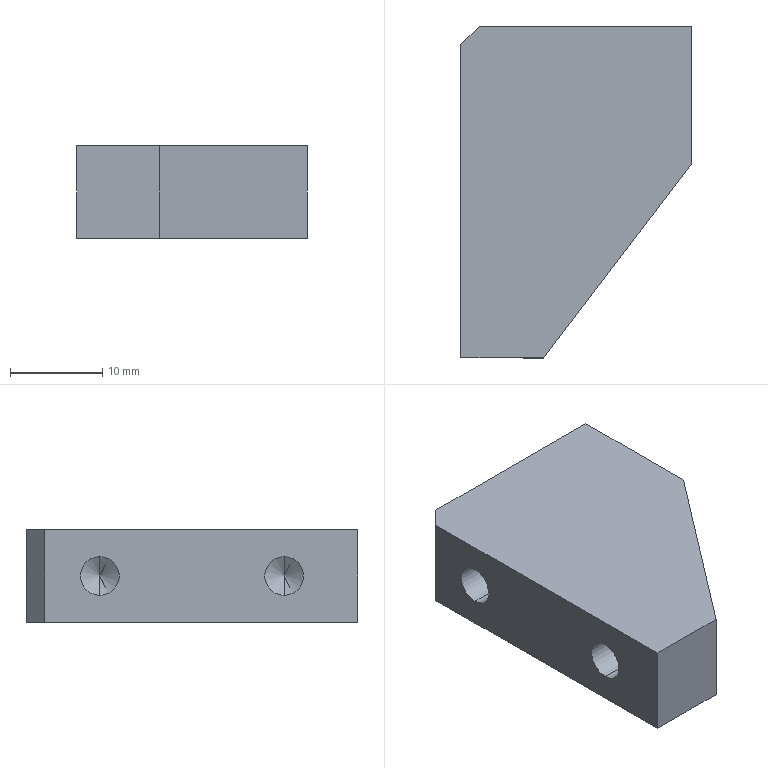Part | SolidWorks | features HoleWzd 2, Chamfer 1, Extrusion 1 | 1 solid | 20 faces | box 25 x 36 x 10 mm | volume 6742 mm3 | plane 8 | cylinder 6 | cone 6 | commonest cylinder face diameters 4.2 x6
STEP:
#1=CARTESIAN_POINT('',(-51.634,-18.797,2.9));
#2=VERTEX_POINT('',#1);
#3=CARTESIAN_POINT('',(-51.634,-18.797,7.1));
#4=VERTEX_POINT('',#3);
#5=CARTESIAN_POINT('',(-51.634,-18.797,5.));
#6=DIRECTION('',(-1.,0.,0.));
#7=DIRECTION('',(0.,0.,1.));
#8=AXIS2_PLACEMENT_3D('',#5,#6,#7);
#9=CIRCLE('',#8,2.1);
#10=EDGE_CURVE('',#2,#4,#9,.T.);
#11=ORIENTED_EDGE('',*,*,#10,.F.);
#12=CARTESIAN_POINT('',(-64.634,-18.797,2.9));
#13=VERTEX_POINT('',#12);
#14=CARTESIAN_POINT('',(-64.634,-18.797,2.9));
#15=DIRECTION('',(-1.,0.,0.));
#16=VECTOR('',#15,1000.);
#17=LINE('',#14,#16);
#18=EDGE_CURVE('',#2,#13,#17,.T.);
#19=ORIENTED_EDGE('',*,*,#18,.T.);
#20=CARTESIAN_POINT('',(-64.634,-18.797,7.1));
#21=VERTEX_POINT('',#20);
#22=CARTESIAN_POINT('',(-64.634,-18.797,5.));
#23=DIRECTION('',(-1.,0.,0.));
#24=DIRECTION('',(0.,0.,1.));
#25=AXIS2_PLACEMENT_3D('',#22,#23,#24);
#26=CIRCLE('',#25,2.1);
#27=EDGE_CURVE('',#13,#21,#26,.T.);
#28=ORIENTED_EDGE('',*,*,#27,.T.);
#29=CARTESIAN_POINT('',(-64.634,-18.797,7.1));
#30=DIRECTION('',(-1.,0.,0.));
#31=VECTOR('',#30,1000.);
#32=LINE('',#29,#31);
#33=EDGE_CURVE('',#4,#21,#32,.T.);
#34=ORIENTED_EDGE('',*,*,#33,.F.);
#35=EDGE_LOOP('',(#11,#19,#28,#34));
#36=FACE_OUTER_BOUND('',#35,.T.);
#37=CARTESIAN_POINT('',(-64.634,-18.797,5.));
#38=DIRECTION('',(-1.,0.,0.));
#39=DIRECTION('',(0.,0.,1.));
#40=AXIS2_PLACEMENT_3D('',#37,#38,#39);
#41=CYLINDRICAL_SURFACE('',#40,2.1);
#42=ADVANCED_FACE('',(#36),#41,.F.);
#43=CARTESIAN_POINT('',(-50.372,-18.797,5.));
#44=VERTEX_POINT('',#43);
#45=CARTESIAN_POINT('',(-51.634,-18.797,7.1));
#46=DIRECTION('',(-0.515,0.,0.8572));
#47=VECTOR('',#46,1000.);
#48=LINE('',#45,#47);
#49=EDGE_CURVE('',#44,#4,#48,.T.);
#50=ORIENTED_EDGE('',*,*,#49,.F.);
#51=CARTESIAN_POINT('',(-51.634,-18.797,2.9));
#52=DIRECTION('',(-0.515,0.,-0.8572));
#53=VECTOR('',#52,1000.);
#54=LINE('',#51,#53);
#55=EDGE_CURVE('',#44,#2,#54,.T.);
#56=ORIENTED_EDGE('',*,*,#55,.T.);
#57=ORIENTED_EDGE('',*,*,#10,.T.);
#58=EDGE_LOOP('',(#50,#56,#57));
#59=FACE_OUTER_BOUND('',#58,.T.);
#60=CARTESIAN_POINT('',(-51.634,-18.797,5.));
#61=DIRECTION('',(-1.,0.,0.));
#62=DIRECTION('',(0.,0.,1.));
#63=AXIS2_PLACEMENT_3D('',#60,#61,#62);
#64=CONICAL_SURFACE('',#63,2.1,1.03);
#65=ADVANCED_FACE('',(#59),#64,.F.);
#66=CARTESIAN_POINT('',(-51.634,-38.797,2.9));
#67=VERTEX_POINT('',#66);
#68=CARTESIAN_POINT('',(-51.634,-38.797,7.1));
#69=VERTEX_POINT('',#68);
#70=CARTESIAN_POINT('',(-51.634,-38.797,5.));
#71=DIRECTION('',(-1.,0.,0.));
#72=DIRECTION('',(0.,0.,1.));
#73=AXIS2_PLACEMENT_3D('',#70,#71,#72);
#74=CIRCLE('',#73,2.1);
#75=EDGE_CURVE('',#67,#69,#74,.T.);
#76=ORIENTED_EDGE('',*,*,#75,.F.);
#77=CARTESIAN_POINT('',(-64.634,-38.797,2.9));
#78=VERTEX_POINT('',#77);
#79=CARTESIAN_POINT('',(-64.634,-38.797,2.9));
#80=DIRECTION('',(-1.,0.,0.));
#81=VECTOR('',#80,1000.);
#82=LINE('',#79,#81);
#83=EDGE_CURVE('',#67,#78,#82,.T.);
#84=ORIENTED_EDGE('',*,*,#83,.T.);
#85=CARTESIAN_POINT('',(-64.634,-38.797,7.1));
#86=VERTEX_POINT('',#85);
#87=CARTESIAN_POINT('',(-64.634,-38.797,5.));
#88=DIRECTION('',(-1.,0.,0.));
#89=DIRECTION('',(0.,0.,1.));
#90=AXIS2_PLACEMENT_3D('',#87,#88,#89);
#91=CIRCLE('',#90,2.1);
#92=EDGE_CURVE('',#78,#86,#91,.T.);
#93=ORIENTED_EDGE('',*,*,#92,.T.);
#94=CARTESIAN_POINT('',(-64.634,-38.797,7.1));
#95=DIRECTION('',(-1.,0.,0.));
#96=VECTOR('',#95,1000.);
#97=LINE('',#94,#96);
#98=EDGE_CURVE('',#69,#86,#97,.T.);
#99=ORIENTED_EDGE('',*,*,#98,.F.);
#100=EDGE_LOOP('',(#76,#84,#93,#99));
#101=FACE_OUTER_BOUND('',#100,.T.);
#102=CARTESIAN_POINT('',(-64.634,-38.797,5.));
#103=DIRECTION('',(-1.,0.,0.));
#104=DIRECTION('',(0.,0.,1.));
#105=AXIS2_PLACEMENT_3D('',#102,#103,#104);
#106=CYLINDRICAL_SURFACE('',#105,2.1);
#107=ADVANCED_FACE('',(#101),#106,.F.);
#108=CARTESIAN_POINT('',(-50.372,-38.797,5.));
#109=VERTEX_POINT('',#108);
#110=CARTESIAN_POINT('',(-51.634,-38.797,7.1));
#111=DIRECTION('',(-0.515,0.,0.8572));
#112=VECTOR('',#111,1000.);
#113=LINE('',#110,#112);
#114=EDGE_CURVE('',#109,#69,#113,.T.);
#115=ORIENTED_EDGE('',*,*,#114,.F.);
#116=CARTESIAN_POINT('',(-51.634,-38.797,2.9));
#117=DIRECTION('',(-0.515,0.,-0.8572));
#118=VECTOR('',#117,1000.);
#119=LINE('',#116,#118);
#120=EDGE_CURVE('',#109,#67,#119,.T.);
#121=ORIENTED_EDGE('',*,*,#120,.T.);
#122=ORIENTED_EDGE('',*,*,#75,.T.);
#123=EDGE_LOOP('',(#115,#121,#122));
#124=FACE_OUTER_BOUND('',#123,.T.);
#125=CARTESIAN_POINT('',(-51.634,-38.797,5.));
#126=DIRECTION('',(-1.,0.,0.));
#127=DIRECTION('',(0.,0.,1.));
#128=AXIS2_PLACEMENT_3D('',#125,#126,#127);
#129=CONICAL_SURFACE('',#128,2.1,1.03);
#130=ADVANCED_FACE('',(#124),#129,.F.);
#131=CARTESIAN_POINT('',(-47.634,-23.797,2.9));
#132=VERTEX_POINT('',#131);
#133=CARTESIAN_POINT('',(-47.634,-23.797,7.1));
#134=VERTEX_POINT('',#133);
#135=CARTESIAN_POINT('',(-47.634,-23.797,5.));
#136=DIRECTION('',(0.,1.,0.));
#137=DIRECTION('',(0.,0.,1.));
#138=AXIS2_PLACEMENT_3D('',#135,#136,#137);
#139=CIRCLE('',#138,2.1);
#140=EDGE_CURVE('',#132,#134,#139,.T.);
#141=ORIENTED_EDGE('',*,*,#140,.F.);
#142=CARTESIAN_POINT('',(-47.634,-10.797,2.9));
#143=VERTEX_POINT('',#142);
#144=CARTESIAN_POINT('',(-47.634,-10.797,2.9));
#145=DIRECTION('',(0.,1.,0.));
#146=VECTOR('',#145,1000.);
#147=LINE('',#144,#146);
#148=EDGE_CURVE('',#132,#143,#147,.T.);
#149=ORIENTED_EDGE('',*,*,#148,.T.);
#150=CARTESIAN_POINT('',(-47.634,-10.797,7.1));
#151=VERTEX_POINT('',#150);
#152=CARTESIAN_POINT('',(-47.634,-10.797,5.));
#153=DIRECTION('',(0.,1.,0.));
#154=DIRECTION('',(0.,0.,1.));
#155=AXIS2_PLACEMENT_3D('',#152,#153,#154);
#156=CIRCLE('',#155,2.1);
#157=EDGE_CURVE('',#143,#151,#156,.T.);
#158=ORIENTED_EDGE('',*,*,#157,.T.);
#159=CARTESIAN_POINT('',(-47.634,-10.797,7.1));
#160=DIRECTION('',(0.,1.,0.));
#161=VECTOR('',#160,1000.);
#162=LINE('',#159,#161);
#163=EDGE_CURVE('',#134,#151,#162,.T.);
#164=ORIENTED_EDGE('',*,*,#163,.F.);
#165=EDGE_LOOP('',(#141,#149,#158,#164));
#166=FACE_OUTER_BOUND('',#165,.T.);
#167=CARTESIAN_POINT('',(-47.634,-10.797,5.));
#168=DIRECTION('',(0.,1.,0.));
#169=DIRECTION('',(0.,0.,1.));
#170=AXIS2_PLACEMENT_3D('',#167,#168,#169);
#171=CYLINDRICAL_SURFACE('',#170,2.1);
#172=ADVANCED_FACE('',(#166),#171,.F.);
#173=CARTESIAN_POINT('',(-47.634,-25.059,5.));
#174=VERTEX_POINT('',#173);
#175=CARTESIAN_POINT('',(-47.634,-23.797,7.1));
#176=DIRECTION('',(0.,0.515,0.8572));
#177=VECTOR('',#176,1000.);
#178=LINE('',#175,#177);
#179=EDGE_CURVE('',#174,#134,#178,.T.);
#180=ORIENTED_EDGE('',*,*,#179,.F.);
#181=CARTESIAN_POINT('',(-47.634,-23.797,2.9));
#182=DIRECTION('',(0.,0.515,-0.8572));
#183=VECTOR('',#182,1000.);
#184=LINE('',#181,#183);
#185=EDGE_CURVE('',#174,#132,#184,.T.);
#186=ORIENTED_EDGE('',*,*,#185,.T.);
#187=ORIENTED_EDGE('',*,*,#140,.T.);
#188=EDGE_LOOP('',(#180,#186,#187));
#189=FACE_OUTER_BOUND('',#188,.T.);
#190=CARTESIAN_POINT('',(-47.634,-23.797,5.));
#191=DIRECTION('',(0.,1.,0.));
#192=DIRECTION('',(0.,0.,1.));
#193=AXIS2_PLACEMENT_3D('',#190,#191,#192);
#194=CONICAL_SURFACE('',#193,2.1,1.03);
#195=ADVANCED_FACE('',(#189),#194,.F.);
#196=CARTESIAN_POINT('',(-64.634,-18.797,5.));
#197=DIRECTION('',(-1.,0.,0.));
#198=DIRECTION('',(0.,0.,1.));
#199=AXIS2_PLACEMENT_3D('',#196,#197,#198);
#200=CIRCLE('',#199,2.1);
#201=EDGE_CURVE('',#21,#13,#200,.T.);
#202=ORIENTED_EDGE('',*,*,#201,.F.);
#203=ORIENTED_EDGE('',*,*,#27,.F.);
#204=EDGE_LOOP('',(#202,#203));
#205=FACE_BOUND('',#204,.T.);
#206=CARTESIAN_POINT('',(-64.634,-38.797,5.));
#207=DIRECTION('',(-1.,0.,0.));
#208=DIRECTION('',(0.,0.,1.));
#209=AXIS2_PLACEMENT_3D('',#206,#207,#208);
#210=CIRCLE('',#209,2.1);
#211=EDGE_CURVE('',#86,#78,#210,.T.);
#212=ORIENTED_EDGE('',*,*,#211,.F.);
#213=ORIENTED_EDGE('',*,*,#92,.F.);
#214=EDGE_LOOP('',(#212,#213));
#215=FACE_BOUND('',#214,.T.);
#216=CARTESIAN_POINT('',(-64.634,-12.797,10.));
#217=VERTEX_POINT('',#216);
#218=CARTESIAN_POINT('',(-64.634,-46.797,10.));
#219=VERTEX_POINT('',#218);
#220=CARTESIAN_POINT('',(-64.634,-10.797,10.));
#221=DIRECTION('',(0.,-1.,0.));
#222=VECTOR('',#221,1000.);
#223=LINE('',#220,#222);
#224=EDGE_CURVE('',#217,#219,#223,.T.);
#225=ORIENTED_EDGE('',*,*,#224,.F.);
#226=CARTESIAN_POINT('',(-64.634,-12.797,0.));
#227=VERTEX_POINT('',#226);
#228=CARTESIAN_POINT('',(-64.634,-12.797,10.));
#229=DIRECTION('',(0.,0.,-1.));
#230=VECTOR('',#229,1000.);
#231=LINE('',#228,#230);
#232=EDGE_CURVE('',#217,#227,#231,.T.);
#233=ORIENTED_EDGE('',*,*,#232,.T.);
#234=CARTESIAN_POINT('',(-64.634,-46.797,0.));
#235=VERTEX_POINT('',#234);
#236=CARTESIAN_POINT('',(-64.634,-10.797,0.));
#237=DIRECTION('',(0.,-1.,0.));
#238=VECTOR('',#237,1000.);
#239=LINE('',#236,#238);
#240=EDGE_CURVE('',#227,#235,#239,.T.);
#241=ORIENTED_EDGE('',*,*,#240,.T.);
#242=CARTESIAN_POINT('',(-64.634,-46.797,10.));
#243=DIRECTION('',(0.,0.,-1.));
#244=VECTOR('',#243,1000.);
#245=LINE('',#242,#244);
#246=EDGE_CURVE('',#219,#235,#245,.T.);
#247=ORIENTED_EDGE('',*,*,#246,.F.);
#248=EDGE_LOOP('',(#225,#233,#241,#247));
#249=FACE_OUTER_BOUND('',#248,.T.);
#250=CARTESIAN_POINT('',(-64.634,-10.797,10.));
#251=DIRECTION('',(1.,0.,0.));
#252=DIRECTION('',(0.,1.,0.));
#253=AXIS2_PLACEMENT_3D('',#250,#251,#252);
#254=PLANE('',#253);
#255=ADVANCED_FACE('',(#205,#215,#249),#254,.F.);
#256=CARTESIAN_POINT('',(-55.634,-46.797,0.));
#257=VERTEX_POINT('',#256);
#258=CARTESIAN_POINT('',(-55.634,-46.797,0.));
#259=DIRECTION('',(1.,0.,0.));
#260=VECTOR('',#259,1000.);
#261=LINE('',#258,#260);
#262=EDGE_CURVE('',#235,#257,#261,.T.);
#263=ORIENTED_EDGE('',*,*,#262,.T.);
#264=CARTESIAN_POINT('',(-55.634,-46.797,10.));
#265=VERTEX_POINT('',#264);
#266=CARTESIAN_POINT('',(-55.634,-46.797,10.));
#267=DIRECTION('',(0.,0.,-1.));
#268=VECTOR('',#267,1000.);
#269=LINE('',#266,#268);
#270=EDGE_CURVE('',#265,#257,#269,.T.);
#271=ORIENTED_EDGE('',*,*,#270,.F.);
#272=CARTESIAN_POINT('',(-55.634,-46.797,10.));
#273=DIRECTION('',(1.,0.,0.));
#274=VECTOR('',#273,1000.);
#275=LINE('',#272,#274);
#276=EDGE_CURVE('',#219,#265,#275,.T.);
#277=ORIENTED_EDGE('',*,*,#276,.F.);
#278=ORIENTED_EDGE('',*,*,#246,.T.);
#279=EDGE_LOOP('',(#263,#271,#277,#278));
#280=FACE_OUTER_BOUND('',#279,.T.);
#281=CARTESIAN_POINT('',(-55.634,-46.797,10.));
#282=DIRECTION('',(0.,1.,0.));
#283=DIRECTION('',(-1.,0.,0.));
#284=AXIS2_PLACEMENT_3D('',#281,#282,#283);
#285=PLANE('',#284);
#286=ADVANCED_FACE('',(#280),#285,.F.);
#287=CARTESIAN_POINT('',(-39.634,-25.797,0.));
#288=VERTEX_POINT('',#287);
#289=CARTESIAN_POINT('',(-39.634,-25.797,0.));
#290=DIRECTION('',(0.606,0.7954,0.));
#291=VECTOR('',#290,1000.);
#292=LINE('',#289,#291);
#293=EDGE_CURVE('',#257,#288,#292,.T.);
#294=ORIENTED_EDGE('',*,*,#293,.T.);
#295=CARTESIAN_POINT('',(-39.634,-25.797,10.));
#296=VERTEX_POINT('',#295);
#297=CARTESIAN_POINT('',(-39.634,-25.797,10.));
#298=DIRECTION('',(0.,0.,-1.));
#299=VECTOR('',#298,1000.);
#300=LINE('',#297,#299);
#301=EDGE_CURVE('',#296,#288,#300,.T.);
#302=ORIENTED_EDGE('',*,*,#301,.F.);
#303=CARTESIAN_POINT('',(-39.634,-25.797,10.));
#304=DIRECTION('',(0.606,0.7954,0.));
#305=VECTOR('',#304,1000.);
#306=LINE('',#303,#305);
#307=EDGE_CURVE('',#265,#296,#306,.T.);
#308=ORIENTED_EDGE('',*,*,#307,.F.);
#309=ORIENTED_EDGE('',*,*,#270,.T.);
#310=EDGE_LOOP('',(#294,#302,#308,#309));
#311=FACE_OUTER_BOUND('',#310,.T.);
#312=CARTESIAN_POINT('',(-39.634,-25.797,10.));
#313=DIRECTION('',(-0.7954,0.606,0.));
#314=DIRECTION('',(-0.606,-0.7954,0.));
#315=AXIS2_PLACEMENT_3D('',#312,#313,#314);
#316=PLANE('',#315);
#317=ADVANCED_FACE('',(#311),#316,.F.);
#318=CARTESIAN_POINT('',(-39.634,-10.797,0.));
#319=VERTEX_POINT('',#318);
#320=CARTESIAN_POINT('',(-39.634,-10.797,0.));
#321=DIRECTION('',(0.,1.,0.));
#322=VECTOR('',#321,1000.);
#323=LINE('',#320,#322);
#324=EDGE_CURVE('',#288,#319,#323,.T.);
#325=ORIENTED_EDGE('',*,*,#324,.T.);
#326=CARTESIAN_POINT('',(-39.634,-10.797,10.));
#327=VERTEX_POINT('',#326);
#328=CARTESIAN_POINT('',(-39.634,-10.797,10.));
#329=DIRECTION('',(0.,0.,-1.));
#330=VECTOR('',#329,1000.);
#331=LINE('',#328,#330);
#332=EDGE_CURVE('',#327,#319,#331,.T.);
#333=ORIENTED_EDGE('',*,*,#332,.F.);
#334=CARTESIAN_POINT('',(-39.634,-10.797,10.));
#335=DIRECTION('',(0.,1.,0.));
#336=VECTOR('',#335,1000.);
#337=LINE('',#334,#336);
#338=EDGE_CURVE('',#296,#327,#337,.T.);
#339=ORIENTED_EDGE('',*,*,#338,.F.);
#340=ORIENTED_EDGE('',*,*,#301,.T.);
#341=EDGE_LOOP('',(#325,#333,#339,#340));
#342=FACE_OUTER_BOUND('',#341,.T.);
#343=CARTESIAN_POINT('',(-39.634,-10.797,10.));
#344=DIRECTION('',(-1.,0.,0.));
#345=DIRECTION('',(0.,0.,1.));
#346=AXIS2_PLACEMENT_3D('',#343,#344,#345);
#347=PLANE('',#346);
#348=ADVANCED_FACE('',(#342),#347,.F.);
#349=CARTESIAN_POINT('',(-47.634,-10.797,5.));
#350=DIRECTION('',(0.,1.,0.));
#351=DIRECTION('',(0.,0.,1.));
#352=AXIS2_PLACEMENT_3D('',#349,#350,#351);
#353=CIRCLE('',#352,2.1);
#354=EDGE_CURVE('',#151,#143,#353,.T.);
#355=ORIENTED_EDGE('',*,*,#354,.F.);
#356=ORIENTED_EDGE('',*,*,#157,.F.);
#357=EDGE_LOOP('',(#355,#356));
#358=FACE_BOUND('',#357,.T.);
#359=CARTESIAN_POINT('',(-62.634,-10.797,0.));
#360=VERTEX_POINT('',#359);
#361=CARTESIAN_POINT('',(-64.634,-10.797,0.));
#362=DIRECTION('',(-1.,0.,0.));
#363=VECTOR('',#362,1000.);
#364=LINE('',#361,#363);
#365=EDGE_CURVE('',#319,#360,#364,.T.);
#366=ORIENTED_EDGE('',*,*,#365,.T.);
#367=CARTESIAN_POINT('',(-62.634,-10.797,10.));
#368=VERTEX_POINT('',#367);
#369=CARTESIAN_POINT('',(-62.634,-10.797,10.));
#370=DIRECTION('',(0.,0.,1.));
#371=VECTOR('',#370,1000.);
#372=LINE('',#369,#371);
#373=EDGE_CURVE('',#360,#368,#372,.T.);
#374=ORIENTED_EDGE('',*,*,#373,.T.);
#375=CARTESIAN_POINT('',(-64.634,-10.797,10.));
#376=DIRECTION('',(-1.,0.,0.));
#377=VECTOR('',#376,1000.);
#378=LINE('',#375,#377);
#379=EDGE_CURVE('',#327,#368,#378,.T.);
#380=ORIENTED_EDGE('',*,*,#379,.F.);
#381=ORIENTED_EDGE('',*,*,#332,.T.);
#382=EDGE_LOOP('',(#366,#374,#380,#381));
#383=FACE_OUTER_BOUND('',#382,.T.);
#384=CARTESIAN_POINT('',(-64.634,-10.797,10.));
#385=DIRECTION('',(0.,-1.,0.));
#386=DIRECTION('',(0.,0.,-1.));
#387=AXIS2_PLACEMENT_3D('',#384,#385,#386);
#388=PLANE('',#387);
#389=ADVANCED_FACE('',(#358,#383),#388,.F.);
#390=ORIENTED_EDGE('',*,*,#379,.T.);
#391=CARTESIAN_POINT('',(-64.634,-12.797,10.));
#392=DIRECTION('',(-0.7071,-0.7071,0.));
#393=VECTOR('',#392,1000.);
#394=LINE('',#391,#393);
#395=EDGE_CURVE('',#368,#217,#394,.T.);
#396=ORIENTED_EDGE('',*,*,#395,.T.);
#397=ORIENTED_EDGE('',*,*,#224,.T.);
#398=ORIENTED_EDGE('',*,*,#276,.T.);
#399=ORIENTED_EDGE('',*,*,#307,.T.);
#400=ORIENTED_EDGE('',*,*,#338,.T.);
#401=EDGE_LOOP('',(#390,#396,#397,#398,#399,#400));
#402=FACE_OUTER_BOUND('',#401,.T.);
#403=CARTESIAN_POINT('',(0.,0.,10.));
#404=DIRECTION('',(0.,0.,-1.));
#405=DIRECTION('',(-1.,0.,0.));
#406=AXIS2_PLACEMENT_3D('',#403,#404,#405);
#407=PLANE('',#406);
#408=ADVANCED_FACE('',(#402),#407,.F.);
#409=ORIENTED_EDGE('',*,*,#240,.F.);
#410=CARTESIAN_POINT('',(-25.919,25.919,0.));
#411=DIRECTION('',(0.7071,0.7071,0.));
#412=VECTOR('',#411,1000.);
#413=LINE('',#410,#412);
#414=EDGE_CURVE('',#227,#360,#413,.T.);
#415=ORIENTED_EDGE('',*,*,#414,.T.);
#416=ORIENTED_EDGE('',*,*,#365,.F.);
#417=ORIENTED_EDGE('',*,*,#324,.F.);
#418=ORIENTED_EDGE('',*,*,#293,.F.);
#419=ORIENTED_EDGE('',*,*,#262,.F.);
#420=EDGE_LOOP('',(#409,#415,#416,#417,#418,#419));
#421=FACE_OUTER_BOUND('',#420,.T.);
#422=CARTESIAN_POINT('',(0.,0.,0.));
#423=DIRECTION('',(0.,0.,-1.));
#424=DIRECTION('',(-1.,0.,0.));
#425=AXIS2_PLACEMENT_3D('',#422,#423,#424);
#426=PLANE('',#425);
#427=ADVANCED_FACE('',(#421),#426,.T.);
#428=ORIENTED_EDGE('',*,*,#185,.F.);
#429=ORIENTED_EDGE('',*,*,#179,.T.);
#430=CARTESIAN_POINT('',(-47.634,-23.797,5.));
#431=DIRECTION('',(0.,1.,0.));
#432=DIRECTION('',(0.,0.,1.));
#433=AXIS2_PLACEMENT_3D('',#430,#431,#432);
#434=CIRCLE('',#433,2.1);
#435=EDGE_CURVE('',#134,#132,#434,.T.);
#436=ORIENTED_EDGE('',*,*,#435,.T.);
#437=EDGE_LOOP('',(#428,#429,#436));
#438=FACE_OUTER_BOUND('',#437,.T.);
#439=CARTESIAN_POINT('',(-47.634,-23.797,5.));
#440=DIRECTION('',(0.,1.,0.));
#441=DIRECTION('',(0.,0.,1.));
#442=AXIS2_PLACEMENT_3D('',#439,#440,#441);
#443=CONICAL_SURFACE('',#442,2.1,1.03);
#444=ADVANCED_FACE('',(#438),#443,.F.);
#445=ORIENTED_EDGE('',*,*,#148,.F.);
#446=ORIENTED_EDGE('',*,*,#435,.F.);
#447=ORIENTED_EDGE('',*,*,#163,.T.);
#448=ORIENTED_EDGE('',*,*,#354,.T.);
#449=EDGE_LOOP('',(#445,#446,#447,#448));
#450=FACE_OUTER_BOUND('',#449,.T.);
#451=CARTESIAN_POINT('',(-47.634,-10.797,5.));
#452=DIRECTION('',(0.,1.,0.));
#453=DIRECTION('',(0.,0.,1.));
#454=AXIS2_PLACEMENT_3D('',#451,#452,#453);
#455=CYLINDRICAL_SURFACE('',#454,2.1);
#456=ADVANCED_FACE('',(#450),#455,.F.);
#457=ORIENTED_EDGE('',*,*,#120,.F.);
#458=ORIENTED_EDGE('',*,*,#114,.T.);
#459=CARTESIAN_POINT('',(-51.634,-38.797,5.));
#460=DIRECTION('',(-1.,0.,0.));
#461=DIRECTION('',(0.,0.,1.));
#462=AXIS2_PLACEMENT_3D('',#459,#460,#461);
#463=CIRCLE('',#462,2.1);
#464=EDGE_CURVE('',#69,#67,#463,.T.);
#465=ORIENTED_EDGE('',*,*,#464,.T.);
#466=EDGE_LOOP('',(#457,#458,#465));
#467=FACE_OUTER_BOUND('',#466,.T.);
#468=CARTESIAN_POINT('',(-51.634,-38.797,5.));
#469=DIRECTION('',(-1.,0.,0.));
#470=DIRECTION('',(0.,0.,1.));
#471=AXIS2_PLACEMENT_3D('',#468,#469,#470);
#472=CONICAL_SURFACE('',#471,2.1,1.03);
#473=ADVANCED_FACE('',(#467),#472,.F.);
#474=ORIENTED_EDGE('',*,*,#83,.F.);
#475=ORIENTED_EDGE('',*,*,#464,.F.);
#476=ORIENTED_EDGE('',*,*,#98,.T.);
#477=ORIENTED_EDGE('',*,*,#211,.T.);
#478=EDGE_LOOP('',(#474,#475,#476,#477));
#479=FACE_OUTER_BOUND('',#478,.T.);
#480=CARTESIAN_POINT('',(-64.634,-38.797,5.));
#481=DIRECTION('',(-1.,0.,0.));
#482=DIRECTION('',(0.,0.,1.));
#483=AXIS2_PLACEMENT_3D('',#480,#481,#482);
#484=CYLINDRICAL_SURFACE('',#483,2.1);
#485=ADVANCED_FACE('',(#479),#484,.F.);
#486=ORIENTED_EDGE('',*,*,#55,.F.);
#487=ORIENTED_EDGE('',*,*,#49,.T.);
#488=CARTESIAN_POINT('',(-51.634,-18.797,5.));
#489=DIRECTION('',(-1.,0.,0.));
#490=DIRECTION('',(0.,0.,1.));
#491=AXIS2_PLACEMENT_3D('',#488,#489,#490);
#492=CIRCLE('',#491,2.1);
#493=EDGE_CURVE('',#4,#2,#492,.T.);
#494=ORIENTED_EDGE('',*,*,#493,.T.);
#495=EDGE_LOOP('',(#486,#487,#494));
#496=FACE_OUTER_BOUND('',#495,.T.);
#497=CARTESIAN_POINT('',(-51.634,-18.797,5.));
#498=DIRECTION('',(-1.,0.,0.));
#499=DIRECTION('',(0.,0.,1.));
#500=AXIS2_PLACEMENT_3D('',#497,#498,#499);
#501=CONICAL_SURFACE('',#500,2.1,1.03);
#502=ADVANCED_FACE('',(#496),#501,.F.);
#503=ORIENTED_EDGE('',*,*,#18,.F.);
#504=ORIENTED_EDGE('',*,*,#493,.F.);
#505=ORIENTED_EDGE('',*,*,#33,.T.);
#506=ORIENTED_EDGE('',*,*,#201,.T.);
#507=EDGE_LOOP('',(#503,#504,#505,#506));
#508=FACE_OUTER_BOUND('',#507,.T.);
#509=CARTESIAN_POINT('',(-64.634,-18.797,5.));
#510=DIRECTION('',(-1.,0.,0.));
#511=DIRECTION('',(0.,0.,1.));
#512=AXIS2_PLACEMENT_3D('',#509,#510,#511);
#513=CYLINDRICAL_SURFACE('',#512,2.1);
#514=ADVANCED_FACE('',(#508),#513,.F.);
#515=ORIENTED_EDGE('',*,*,#395,.F.);
#516=ORIENTED_EDGE('',*,*,#373,.F.);
#517=ORIENTED_EDGE('',*,*,#414,.F.);
#518=ORIENTED_EDGE('',*,*,#232,.F.);
#519=EDGE_LOOP('',(#515,#516,#517,#518));
#520=FACE_OUTER_BOUND('',#519,.T.);
#521=CARTESIAN_POINT('',(-64.634,-12.797,10.));
#522=DIRECTION('',(0.7071,-0.7071,0.));
#523=DIRECTION('',(0.,0.,-1.));
#524=AXIS2_PLACEMENT_3D('',#521,#522,#523);
#525=PLANE('',#524);
#526=ADVANCED_FACE('',(#520),#525,.F.);
#527=CLOSED_SHELL('',(#42,#65,#107,#130,#172,#195,#255,#286,#317,#348,#389,#408,#427,#444,#456,#473,#485,#502,#514,#526));
#528=MANIFOLD_SOLID_BREP('',#527);
#529=CARTESIAN_POINT('',(0.,0.,0.));
#530=DIRECTION('',(0.,0.,1.));
#531=DIRECTION('',(1.,0.,0.));
#532=AXIS2_PLACEMENT_3D('',#529,#530,#531);
#533=(LENGTH_UNIT()NAMED_UNIT(*)SI_UNIT(.MILLI.,.METRE.));
#534=UNCERTAINTY_MEASURE_WITH_UNIT(LENGTH_MEASURE(0.00001),#533,'','');
#535=(NAMED_UNIT(*)PLANE_ANGLE_UNIT()SI_UNIT($,.RADIAN.));
#536=(NAMED_UNIT(*)SI_UNIT($,.STERADIAN.)SOLID_ANGLE_UNIT());
#537=(GEOMETRIC_REPRESENTATION_CONTEXT(3)GLOBAL_UNCERTAINTY_ASSIGNED_CONTEXT((#534))GLOBAL_UNIT_ASSIGNED_CONTEXT((#533,#535,#536))REPRESENTATION_CONTEXT('',''));
#538=ADVANCED_BREP_SHAPE_REPRESENTATION('',(#528,#532),#537);